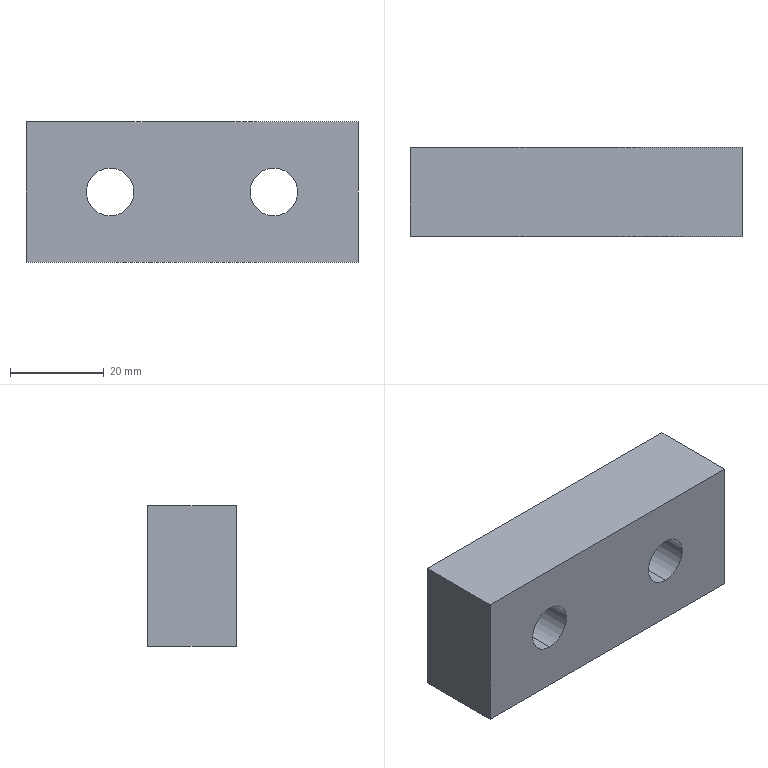Part | SolidWorks | features FlatPattern 1, HoleWzd 1, SMBaseFlange 1, SheetMetal 1 | 1 solid | 10 faces | box 71 x 19 x 30 mm | volume 37365 mm3 | plane 6 | cylinder 4 | commonest cylinder face diameters 10.2 x4
STEP:
#1=CARTESIAN_POINT('',(-17.5,-19.,-5.1));
#2=VERTEX_POINT('',#1);
#3=CARTESIAN_POINT('',(-17.5,-19.,5.1));
#4=VERTEX_POINT('',#3);
#5=CARTESIAN_POINT('',(-17.5,-19.,0.));
#6=DIRECTION('',(0.,1.,0.));
#7=DIRECTION('',(0.,0.,1.));
#8=AXIS2_PLACEMENT_3D('',#5,#6,#7);
#9=CIRCLE('',#8,5.1);
#10=EDGE_CURVE('',#2,#4,#9,.T.);
#11=ORIENTED_EDGE('',*,*,#10,.F.);
#12=CARTESIAN_POINT('',(-17.5,0.,-5.1));
#13=VERTEX_POINT('',#12);
#14=CARTESIAN_POINT('',(-17.5,0.,-5.1));
#15=DIRECTION('',(0.,1.,0.));
#16=VECTOR('',#15,1000.);
#17=LINE('',#14,#16);
#18=EDGE_CURVE('',#2,#13,#17,.T.);
#19=ORIENTED_EDGE('',*,*,#18,.T.);
#20=CARTESIAN_POINT('',(-17.5,0.,5.1));
#21=VERTEX_POINT('',#20);
#22=CARTESIAN_POINT('',(-17.5,0.,0.));
#23=DIRECTION('',(0.,1.,0.));
#24=DIRECTION('',(0.,0.,1.));
#25=AXIS2_PLACEMENT_3D('',#22,#23,#24);
#26=CIRCLE('',#25,5.1);
#27=EDGE_CURVE('',#13,#21,#26,.T.);
#28=ORIENTED_EDGE('',*,*,#27,.T.);
#29=CARTESIAN_POINT('',(-17.5,0.,5.1));
#30=DIRECTION('',(0.,1.,0.));
#31=VECTOR('',#30,1000.);
#32=LINE('',#29,#31);
#33=EDGE_CURVE('',#4,#21,#32,.T.);
#34=ORIENTED_EDGE('',*,*,#33,.F.);
#35=EDGE_LOOP('',(#11,#19,#28,#34));
#36=FACE_OUTER_BOUND('',#35,.T.);
#37=CARTESIAN_POINT('',(-17.5,0.,0.));
#38=DIRECTION('',(0.,1.,0.));
#39=DIRECTION('',(0.,0.,1.));
#40=AXIS2_PLACEMENT_3D('',#37,#38,#39);
#41=CYLINDRICAL_SURFACE('',#40,5.1);
#42=ADVANCED_FACE('',(#36),#41,.F.);
#43=CARTESIAN_POINT('',(17.5,-19.,-5.1));
#44=VERTEX_POINT('',#43);
#45=CARTESIAN_POINT('',(17.5,-19.,5.1));
#46=VERTEX_POINT('',#45);
#47=CARTESIAN_POINT('',(17.5,-19.,0.));
#48=DIRECTION('',(0.,1.,0.));
#49=DIRECTION('',(0.,0.,1.));
#50=AXIS2_PLACEMENT_3D('',#47,#48,#49);
#51=CIRCLE('',#50,5.1);
#52=EDGE_CURVE('',#44,#46,#51,.T.);
#53=ORIENTED_EDGE('',*,*,#52,.F.);
#54=CARTESIAN_POINT('',(17.5,0.,-5.1));
#55=VERTEX_POINT('',#54);
#56=CARTESIAN_POINT('',(17.5,0.,-5.1));
#57=DIRECTION('',(0.,1.,0.));
#58=VECTOR('',#57,1000.);
#59=LINE('',#56,#58);
#60=EDGE_CURVE('',#44,#55,#59,.T.);
#61=ORIENTED_EDGE('',*,*,#60,.T.);
#62=CARTESIAN_POINT('',(17.5,0.,5.1));
#63=VERTEX_POINT('',#62);
#64=CARTESIAN_POINT('',(17.5,0.,0.));
#65=DIRECTION('',(0.,1.,0.));
#66=DIRECTION('',(0.,0.,1.));
#67=AXIS2_PLACEMENT_3D('',#64,#65,#66);
#68=CIRCLE('',#67,5.1);
#69=EDGE_CURVE('',#55,#63,#68,.T.);
#70=ORIENTED_EDGE('',*,*,#69,.T.);
#71=CARTESIAN_POINT('',(17.5,0.,5.1));
#72=DIRECTION('',(0.,1.,0.));
#73=VECTOR('',#72,1000.);
#74=LINE('',#71,#73);
#75=EDGE_CURVE('',#46,#63,#74,.T.);
#76=ORIENTED_EDGE('',*,*,#75,.F.);
#77=EDGE_LOOP('',(#53,#61,#70,#76));
#78=FACE_OUTER_BOUND('',#77,.T.);
#79=CARTESIAN_POINT('',(17.5,0.,0.));
#80=DIRECTION('',(0.,1.,0.));
#81=DIRECTION('',(0.,0.,1.));
#82=AXIS2_PLACEMENT_3D('',#79,#80,#81);
#83=CYLINDRICAL_SURFACE('',#82,5.1);
#84=ADVANCED_FACE('',(#78),#83,.F.);
#85=CARTESIAN_POINT('',(35.5,0.,15.));
#86=VERTEX_POINT('',#85);
#87=CARTESIAN_POINT('',(35.5,0.,-15.));
#88=VERTEX_POINT('',#87);
#89=CARTESIAN_POINT('',(35.5,0.,-15.));
#90=DIRECTION('',(0.,0.,-1.));
#91=VECTOR('',#90,1000.);
#92=LINE('',#89,#91);
#93=EDGE_CURVE('',#86,#88,#92,.T.);
#94=ORIENTED_EDGE('',*,*,#93,.F.);
#95=CARTESIAN_POINT('',(35.5,-19.,15.));
#96=VERTEX_POINT('',#95);
#97=CARTESIAN_POINT('',(35.5,-19.,15.));
#98=DIRECTION('',(0.,1.,0.));
#99=VECTOR('',#98,1000.);
#100=LINE('',#97,#99);
#101=EDGE_CURVE('',#96,#86,#100,.T.);
#102=ORIENTED_EDGE('',*,*,#101,.F.);
#103=CARTESIAN_POINT('',(35.5,-19.,-15.));
#104=VERTEX_POINT('',#103);
#105=CARTESIAN_POINT('',(35.5,-19.,-15.));
#106=DIRECTION('',(0.,0.,-1.));
#107=VECTOR('',#106,1000.);
#108=LINE('',#105,#107);
#109=EDGE_CURVE('',#96,#104,#108,.T.);
#110=ORIENTED_EDGE('',*,*,#109,.T.);
#111=CARTESIAN_POINT('',(35.5,-19.,-15.));
#112=DIRECTION('',(0.,1.,0.));
#113=VECTOR('',#112,1000.);
#114=LINE('',#111,#113);
#115=EDGE_CURVE('',#104,#88,#114,.T.);
#116=ORIENTED_EDGE('',*,*,#115,.T.);
#117=EDGE_LOOP('',(#94,#102,#110,#116));
#118=FACE_OUTER_BOUND('',#117,.T.);
#119=CARTESIAN_POINT('',(35.5,-19.,-15.));
#120=DIRECTION('',(1.,0.,0.));
#121=DIRECTION('',(0.,0.,-1.));
#122=AXIS2_PLACEMENT_3D('',#119,#120,#121);
#123=PLANE('',#122);
#124=ADVANCED_FACE('',(#118),#123,.T.);
#125=CARTESIAN_POINT('',(-35.5,0.,15.));
#126=VERTEX_POINT('',#125);
#127=CARTESIAN_POINT('',(-35.5,0.,15.));
#128=DIRECTION('',(1.,0.,0.));
#129=VECTOR('',#128,1000.);
#130=LINE('',#127,#129);
#131=EDGE_CURVE('',#126,#86,#130,.T.);
#132=ORIENTED_EDGE('',*,*,#131,.F.);
#133=CARTESIAN_POINT('',(-35.5,-19.,15.));
#134=VERTEX_POINT('',#133);
#135=CARTESIAN_POINT('',(-35.5,-19.,15.));
#136=DIRECTION('',(0.,1.,0.));
#137=VECTOR('',#136,1000.);
#138=LINE('',#135,#137);
#139=EDGE_CURVE('',#134,#126,#138,.T.);
#140=ORIENTED_EDGE('',*,*,#139,.F.);
#141=CARTESIAN_POINT('',(-35.5,-19.,15.));
#142=DIRECTION('',(1.,0.,0.));
#143=VECTOR('',#142,1000.);
#144=LINE('',#141,#143);
#145=EDGE_CURVE('',#134,#96,#144,.T.);
#146=ORIENTED_EDGE('',*,*,#145,.T.);
#147=ORIENTED_EDGE('',*,*,#101,.T.);
#148=EDGE_LOOP('',(#132,#140,#146,#147));
#149=FACE_OUTER_BOUND('',#148,.T.);
#150=CARTESIAN_POINT('',(-35.5,-19.,15.));
#151=DIRECTION('',(0.,0.,1.));
#152=DIRECTION('',(1.,0.,0.));
#153=AXIS2_PLACEMENT_3D('',#150,#151,#152);
#154=PLANE('',#153);
#155=ADVANCED_FACE('',(#149),#154,.T.);
#156=CARTESIAN_POINT('',(-35.5,0.,-15.));
#157=VERTEX_POINT('',#156);
#158=CARTESIAN_POINT('',(-35.5,0.,-15.));
#159=DIRECTION('',(0.,0.,1.));
#160=VECTOR('',#159,1000.);
#161=LINE('',#158,#160);
#162=EDGE_CURVE('',#157,#126,#161,.T.);
#163=ORIENTED_EDGE('',*,*,#162,.F.);
#164=CARTESIAN_POINT('',(-35.5,-19.,-15.));
#165=VERTEX_POINT('',#164);
#166=CARTESIAN_POINT('',(-35.5,-19.,-15.));
#167=DIRECTION('',(0.,1.,0.));
#168=VECTOR('',#167,1000.);
#169=LINE('',#166,#168);
#170=EDGE_CURVE('',#165,#157,#169,.T.);
#171=ORIENTED_EDGE('',*,*,#170,.F.);
#172=CARTESIAN_POINT('',(-35.5,-19.,-15.));
#173=DIRECTION('',(0.,0.,1.));
#174=VECTOR('',#173,1000.);
#175=LINE('',#172,#174);
#176=EDGE_CURVE('',#165,#134,#175,.T.);
#177=ORIENTED_EDGE('',*,*,#176,.T.);
#178=ORIENTED_EDGE('',*,*,#139,.T.);
#179=EDGE_LOOP('',(#163,#171,#177,#178));
#180=FACE_OUTER_BOUND('',#179,.T.);
#181=CARTESIAN_POINT('',(-35.5,-19.,-15.));
#182=DIRECTION('',(-1.,0.,0.));
#183=DIRECTION('',(0.,0.,1.));
#184=AXIS2_PLACEMENT_3D('',#181,#182,#183);
#185=PLANE('',#184);
#186=ADVANCED_FACE('',(#180),#185,.T.);
#187=CARTESIAN_POINT('',(-35.5,0.,-15.));
#188=DIRECTION('',(-1.,0.,0.));
#189=VECTOR('',#188,1000.);
#190=LINE('',#187,#189);
#191=EDGE_CURVE('',#88,#157,#190,.T.);
#192=ORIENTED_EDGE('',*,*,#191,.F.);
#193=ORIENTED_EDGE('',*,*,#115,.F.);
#194=CARTESIAN_POINT('',(-35.5,-19.,-15.));
#195=DIRECTION('',(-1.,0.,0.));
#196=VECTOR('',#195,1000.);
#197=LINE('',#194,#196);
#198=EDGE_CURVE('',#104,#165,#197,.T.);
#199=ORIENTED_EDGE('',*,*,#198,.T.);
#200=ORIENTED_EDGE('',*,*,#170,.T.);
#201=EDGE_LOOP('',(#192,#193,#199,#200));
#202=FACE_OUTER_BOUND('',#201,.T.);
#203=CARTESIAN_POINT('',(-35.5,-19.,-15.));
#204=DIRECTION('',(0.,0.,-1.));
#205=DIRECTION('',(-1.,0.,0.));
#206=AXIS2_PLACEMENT_3D('',#203,#204,#205);
#207=PLANE('',#206);
#208=ADVANCED_FACE('',(#202),#207,.T.);
#209=CARTESIAN_POINT('',(-17.5,-19.,0.));
#210=DIRECTION('',(0.,1.,0.));
#211=DIRECTION('',(0.,0.,1.));
#212=AXIS2_PLACEMENT_3D('',#209,#210,#211);
#213=CIRCLE('',#212,5.1);
#214=EDGE_CURVE('',#4,#2,#213,.T.);
#215=ORIENTED_EDGE('',*,*,#214,.T.);
#216=ORIENTED_EDGE('',*,*,#10,.T.);
#217=EDGE_LOOP('',(#215,#216));
#218=FACE_BOUND('',#217,.T.);
#219=CARTESIAN_POINT('',(17.5,-19.,0.));
#220=DIRECTION('',(0.,1.,0.));
#221=DIRECTION('',(0.,0.,1.));
#222=AXIS2_PLACEMENT_3D('',#219,#220,#221);
#223=CIRCLE('',#222,5.1);
#224=EDGE_CURVE('',#46,#44,#223,.T.);
#225=ORIENTED_EDGE('',*,*,#224,.T.);
#226=ORIENTED_EDGE('',*,*,#52,.T.);
#227=EDGE_LOOP('',(#225,#226));
#228=FACE_BOUND('',#227,.T.);
#229=ORIENTED_EDGE('',*,*,#109,.F.);
#230=ORIENTED_EDGE('',*,*,#145,.F.);
#231=ORIENTED_EDGE('',*,*,#176,.F.);
#232=ORIENTED_EDGE('',*,*,#198,.F.);
#233=EDGE_LOOP('',(#229,#230,#231,#232));
#234=FACE_OUTER_BOUND('',#233,.T.);
#235=CARTESIAN_POINT('',(0.,-19.,0.));
#236=DIRECTION('',(0.,1.,0.));
#237=DIRECTION('',(0.,0.,1.));
#238=AXIS2_PLACEMENT_3D('',#235,#236,#237);
#239=PLANE('',#238);
#240=ADVANCED_FACE('',(#218,#228,#234),#239,.F.);
#241=CARTESIAN_POINT('',(-17.5,0.,0.));
#242=DIRECTION('',(0.,1.,0.));
#243=DIRECTION('',(0.,0.,1.));
#244=AXIS2_PLACEMENT_3D('',#241,#242,#243);
#245=CIRCLE('',#244,5.1);
#246=EDGE_CURVE('',#21,#13,#245,.T.);
#247=ORIENTED_EDGE('',*,*,#246,.F.);
#248=ORIENTED_EDGE('',*,*,#27,.F.);
#249=EDGE_LOOP('',(#247,#248));
#250=FACE_BOUND('',#249,.T.);
#251=CARTESIAN_POINT('',(17.5,0.,0.));
#252=DIRECTION('',(0.,1.,0.));
#253=DIRECTION('',(0.,0.,1.));
#254=AXIS2_PLACEMENT_3D('',#251,#252,#253);
#255=CIRCLE('',#254,5.1);
#256=EDGE_CURVE('',#63,#55,#255,.T.);
#257=ORIENTED_EDGE('',*,*,#256,.F.);
#258=ORIENTED_EDGE('',*,*,#69,.F.);
#259=EDGE_LOOP('',(#257,#258));
#260=FACE_BOUND('',#259,.T.);
#261=ORIENTED_EDGE('',*,*,#93,.T.);
#262=ORIENTED_EDGE('',*,*,#191,.T.);
#263=ORIENTED_EDGE('',*,*,#162,.T.);
#264=ORIENTED_EDGE('',*,*,#131,.T.);
#265=EDGE_LOOP('',(#261,#262,#263,#264));
#266=FACE_OUTER_BOUND('',#265,.T.);
#267=CARTESIAN_POINT('',(0.,0.,0.));
#268=DIRECTION('',(0.,1.,0.));
#269=DIRECTION('',(0.,0.,1.));
#270=AXIS2_PLACEMENT_3D('',#267,#268,#269);
#271=PLANE('',#270);
#272=ADVANCED_FACE('',(#250,#260,#266),#271,.T.);
#273=ORIENTED_EDGE('',*,*,#60,.F.);
#274=ORIENTED_EDGE('',*,*,#224,.F.);
#275=ORIENTED_EDGE('',*,*,#75,.T.);
#276=ORIENTED_EDGE('',*,*,#256,.T.);
#277=EDGE_LOOP('',(#273,#274,#275,#276));
#278=FACE_OUTER_BOUND('',#277,.T.);
#279=CARTESIAN_POINT('',(17.5,0.,0.));
#280=DIRECTION('',(0.,1.,0.));
#281=DIRECTION('',(0.,0.,1.));
#282=AXIS2_PLACEMENT_3D('',#279,#280,#281);
#283=CYLINDRICAL_SURFACE('',#282,5.1);
#284=ADVANCED_FACE('',(#278),#283,.F.);
#285=ORIENTED_EDGE('',*,*,#18,.F.);
#286=ORIENTED_EDGE('',*,*,#214,.F.);
#287=ORIENTED_EDGE('',*,*,#33,.T.);
#288=ORIENTED_EDGE('',*,*,#246,.T.);
#289=EDGE_LOOP('',(#285,#286,#287,#288));
#290=FACE_OUTER_BOUND('',#289,.T.);
#291=CARTESIAN_POINT('',(-17.5,0.,0.));
#292=DIRECTION('',(0.,1.,0.));
#293=DIRECTION('',(0.,0.,1.));
#294=AXIS2_PLACEMENT_3D('',#291,#292,#293);
#295=CYLINDRICAL_SURFACE('',#294,5.1);
#296=ADVANCED_FACE('',(#290),#295,.F.);
#297=CLOSED_SHELL('',(#42,#84,#124,#155,#186,#208,#240,#272,#284,#296));
#298=MANIFOLD_SOLID_BREP('',#297);
#299=CARTESIAN_POINT('',(0.,0.,0.));
#300=DIRECTION('',(0.,0.,1.));
#301=DIRECTION('',(1.,0.,0.));
#302=AXIS2_PLACEMENT_3D('',#299,#300,#301);
#303=(LENGTH_UNIT()NAMED_UNIT(*)SI_UNIT(.MILLI.,.METRE.));
#304=UNCERTAINTY_MEASURE_WITH_UNIT(LENGTH_MEASURE(0.00001),#303,'','');
#305=(NAMED_UNIT(*)PLANE_ANGLE_UNIT()SI_UNIT($,.RADIAN.));
#306=(NAMED_UNIT(*)SI_UNIT($,.STERADIAN.)SOLID_ANGLE_UNIT());
#307=(GEOMETRIC_REPRESENTATION_CONTEXT(3)GLOBAL_UNCERTAINTY_ASSIGNED_CONTEXT((#304))GLOBAL_UNIT_ASSIGNED_CONTEXT((#303,#305,#306))REPRESENTATION_CONTEXT('',''));
#308=ADVANCED_BREP_SHAPE_REPRESENTATION('',(#298,#302),#307);